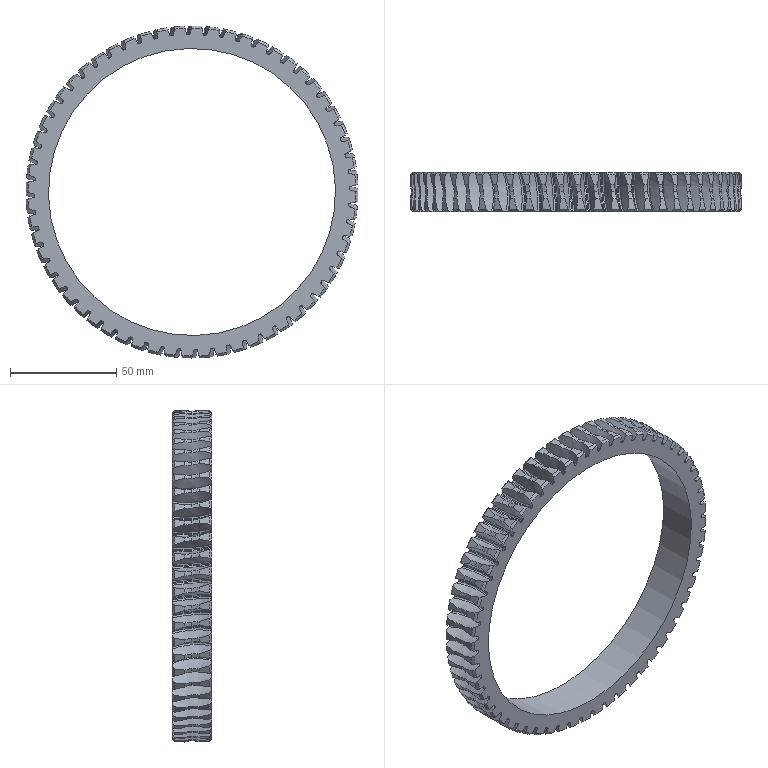Part | STEP file | 2[63] | 1 solid | 723 faces | box 156.134 x 18.5 x 156.134 mm | volume 66300 mm3 | cylinder 241 | spline 240 | torus 120 | cone 120 | plane 2 | commonest cylinder face diameters 156.134 x120 32.695 x119 135 x2